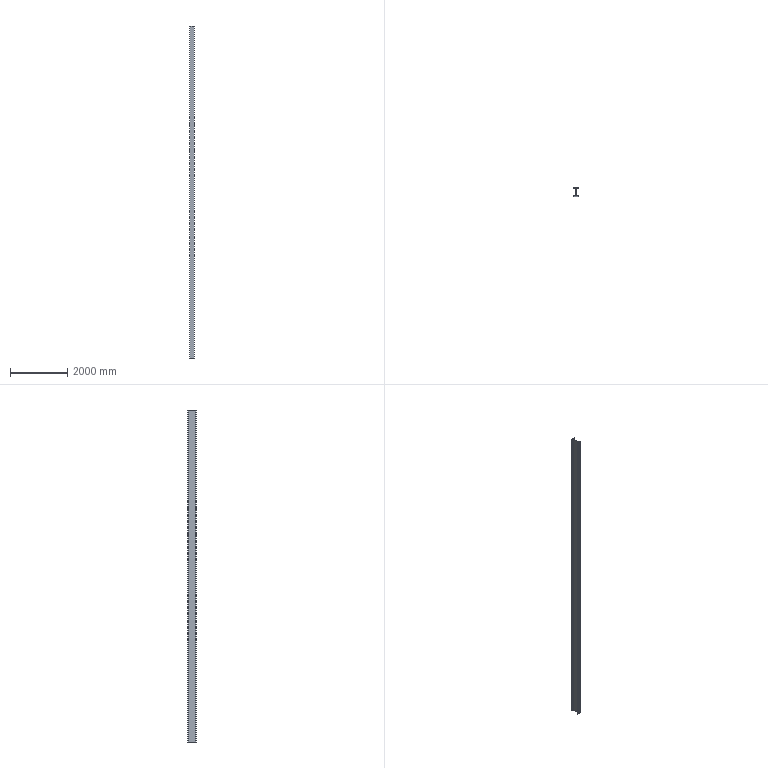Part | SolidWorks | features Extrusion 1 | 1 solid | 18 faces | box 150 x 300 x 11647 mm | volume 54485491 mm3 | plane 14 | cylinder 4 | commonest cylinder face diameters 26 x4
STEP:
#1=CARTESIAN_POINT('',(-75.,9.,0.));
#2=VERTEX_POINT('',#1);
#3=CARTESIAN_POINT('',(-75.,0.,0.));
#4=VERTEX_POINT('',#3);
#5=CARTESIAN_POINT('',(-75.,0.,0.));
#6=DIRECTION('',(0.,-1.,0.));
#7=VECTOR('',#6,1000.);
#8=LINE('',#5,#7);
#9=EDGE_CURVE('',#2,#4,#8,.T.);
#10=ORIENTED_EDGE('',*,*,#9,.T.);
#11=CARTESIAN_POINT('',(-75.,0.,11647.));
#12=VERTEX_POINT('',#11);
#13=CARTESIAN_POINT('',(-75.,0.,11647.));
#14=DIRECTION('',(0.,0.,-1.));
#15=VECTOR('',#14,1000.);
#16=LINE('',#13,#15);
#17=EDGE_CURVE('',#12,#4,#16,.T.);
#18=ORIENTED_EDGE('',*,*,#17,.F.);
#19=CARTESIAN_POINT('',(-75.,9.,11647.));
#20=VERTEX_POINT('',#19);
#21=CARTESIAN_POINT('',(-75.,0.,11647.));
#22=DIRECTION('',(0.,-1.,0.));
#23=VECTOR('',#22,1000.);
#24=LINE('',#21,#23);
#25=EDGE_CURVE('',#20,#12,#24,.T.);
#26=ORIENTED_EDGE('',*,*,#25,.F.);
#27=CARTESIAN_POINT('',(-75.,9.,11647.));
#28=DIRECTION('',(0.,0.,-1.));
#29=VECTOR('',#28,1000.);
#30=LINE('',#27,#29);
#31=EDGE_CURVE('',#20,#2,#30,.T.);
#32=ORIENTED_EDGE('',*,*,#31,.T.);
#33=EDGE_LOOP('',(#10,#18,#26,#32));
#34=FACE_OUTER_BOUND('',#33,.T.);
#35=CARTESIAN_POINT('',(-75.,0.,11647.));
#36=DIRECTION('',(1.,0.,0.));
#37=DIRECTION('',(0.,0.,-1.));
#38=AXIS2_PLACEMENT_3D('',#35,#36,#37);
#39=PLANE('',#38);
#40=ADVANCED_FACE('',(#34),#39,.F.);
#41=CARTESIAN_POINT('',(75.,0.,0.));
#42=VERTEX_POINT('',#41);
#43=CARTESIAN_POINT('',(75.,0.,0.));
#44=DIRECTION('',(1.,0.,0.));
#45=VECTOR('',#44,1000.);
#46=LINE('',#43,#45);
#47=EDGE_CURVE('',#4,#42,#46,.T.);
#48=ORIENTED_EDGE('',*,*,#47,.T.);
#49=CARTESIAN_POINT('',(75.,0.,11647.));
#50=VERTEX_POINT('',#49);
#51=CARTESIAN_POINT('',(75.,0.,11647.));
#52=DIRECTION('',(0.,0.,-1.));
#53=VECTOR('',#52,1000.);
#54=LINE('',#51,#53);
#55=EDGE_CURVE('',#50,#42,#54,.T.);
#56=ORIENTED_EDGE('',*,*,#55,.F.);
#57=CARTESIAN_POINT('',(75.,0.,11647.));
#58=DIRECTION('',(1.,0.,0.));
#59=VECTOR('',#58,1000.);
#60=LINE('',#57,#59);
#61=EDGE_CURVE('',#12,#50,#60,.T.);
#62=ORIENTED_EDGE('',*,*,#61,.F.);
#63=ORIENTED_EDGE('',*,*,#17,.T.);
#64=EDGE_LOOP('',(#48,#56,#62,#63));
#65=FACE_OUTER_BOUND('',#64,.T.);
#66=CARTESIAN_POINT('',(75.,0.,11647.));
#67=DIRECTION('',(0.,1.,0.));
#68=DIRECTION('',(-1.,0.,0.));
#69=AXIS2_PLACEMENT_3D('',#66,#67,#68);
#70=PLANE('',#69);
#71=ADVANCED_FACE('',(#65),#70,.F.);
#72=CARTESIAN_POINT('',(75.,9.,0.));
#73=VERTEX_POINT('',#72);
#74=CARTESIAN_POINT('',(75.,0.,0.));
#75=DIRECTION('',(0.,1.,0.));
#76=VECTOR('',#75,1000.);
#77=LINE('',#74,#76);
#78=EDGE_CURVE('',#42,#73,#77,.T.);
#79=ORIENTED_EDGE('',*,*,#78,.T.);
#80=CARTESIAN_POINT('',(75.,9.,11647.));
#81=VERTEX_POINT('',#80);
#82=CARTESIAN_POINT('',(75.,9.,11647.));
#83=DIRECTION('',(0.,0.,-1.));
#84=VECTOR('',#83,1000.);
#85=LINE('',#82,#84);
#86=EDGE_CURVE('',#81,#73,#85,.T.);
#87=ORIENTED_EDGE('',*,*,#86,.F.);
#88=CARTESIAN_POINT('',(75.,0.,11647.));
#89=DIRECTION('',(0.,1.,0.));
#90=VECTOR('',#89,1000.);
#91=LINE('',#88,#90);
#92=EDGE_CURVE('',#50,#81,#91,.T.);
#93=ORIENTED_EDGE('',*,*,#92,.F.);
#94=ORIENTED_EDGE('',*,*,#55,.T.);
#95=EDGE_LOOP('',(#79,#87,#93,#94));
#96=FACE_OUTER_BOUND('',#95,.T.);
#97=CARTESIAN_POINT('',(75.,0.,11647.));
#98=DIRECTION('',(-1.,0.,0.));
#99=DIRECTION('',(0.,0.,1.));
#100=AXIS2_PLACEMENT_3D('',#97,#98,#99);
#101=PLANE('',#100);
#102=ADVANCED_FACE('',(#96),#101,.F.);
#103=CARTESIAN_POINT('',(16.25,9.,0.));
#104=VERTEX_POINT('',#103);
#105=CARTESIAN_POINT('',(75.,9.,0.));
#106=DIRECTION('',(-1.,0.,0.));
#107=VECTOR('',#106,1000.);
#108=LINE('',#105,#107);
#109=EDGE_CURVE('',#73,#104,#108,.T.);
#110=ORIENTED_EDGE('',*,*,#109,.T.);
#111=CARTESIAN_POINT('',(16.25,9.,11647.));
#112=VERTEX_POINT('',#111);
#113=CARTESIAN_POINT('',(16.25,9.,11647.));
#114=DIRECTION('',(0.,0.,-1.));
#115=VECTOR('',#114,1000.);
#116=LINE('',#113,#115);
#117=EDGE_CURVE('',#112,#104,#116,.T.);
#118=ORIENTED_EDGE('',*,*,#117,.F.);
#119=CARTESIAN_POINT('',(75.,9.,11647.));
#120=DIRECTION('',(-1.,0.,0.));
#121=VECTOR('',#120,1000.);
#122=LINE('',#119,#121);
#123=EDGE_CURVE('',#81,#112,#122,.T.);
#124=ORIENTED_EDGE('',*,*,#123,.F.);
#125=ORIENTED_EDGE('',*,*,#86,.T.);
#126=EDGE_LOOP('',(#110,#118,#124,#125));
#127=FACE_OUTER_BOUND('',#126,.T.);
#128=CARTESIAN_POINT('',(75.,9.,11647.));
#129=DIRECTION('',(0.,-1.,0.));
#130=DIRECTION('',(1.,0.,0.));
#131=AXIS2_PLACEMENT_3D('',#128,#129,#130);
#132=PLANE('',#131);
#133=ADVANCED_FACE('',(#127),#132,.F.);
#134=CARTESIAN_POINT('',(3.25,22.,0.));
#135=VERTEX_POINT('',#134);
#136=CARTESIAN_POINT('',(16.25,22.,0.));
#137=DIRECTION('',(0.,0.,-1.));
#138=DIRECTION('',(-1.,0.,0.));
#139=AXIS2_PLACEMENT_3D('',#136,#137,#138);
#140=CIRCLE('',#139,13.);
#141=EDGE_CURVE('',#104,#135,#140,.T.);
#142=ORIENTED_EDGE('',*,*,#141,.T.);
#143=CARTESIAN_POINT('',(3.25,22.,11647.));
#144=VERTEX_POINT('',#143);
#145=CARTESIAN_POINT('',(3.25,22.,11647.));
#146=DIRECTION('',(0.,0.,-1.));
#147=VECTOR('',#146,1000.);
#148=LINE('',#145,#147);
#149=EDGE_CURVE('',#144,#135,#148,.T.);
#150=ORIENTED_EDGE('',*,*,#149,.F.);
#151=CARTESIAN_POINT('',(16.25,22.,11647.));
#152=DIRECTION('',(0.,0.,-1.));
#153=DIRECTION('',(-1.,0.,0.));
#154=AXIS2_PLACEMENT_3D('',#151,#152,#153);
#155=CIRCLE('',#154,13.);
#156=EDGE_CURVE('',#112,#144,#155,.T.);
#157=ORIENTED_EDGE('',*,*,#156,.F.);
#158=ORIENTED_EDGE('',*,*,#117,.T.);
#159=EDGE_LOOP('',(#142,#150,#157,#158));
#160=FACE_OUTER_BOUND('',#159,.T.);
#161=CARTESIAN_POINT('',(16.25,22.,11647.));
#162=DIRECTION('',(0.,0.,-1.));
#163=DIRECTION('',(-1.,0.,0.));
#164=AXIS2_PLACEMENT_3D('',#161,#162,#163);
#165=CYLINDRICAL_SURFACE('',#164,13.);
#166=ADVANCED_FACE('',(#160),#165,.F.);
#167=CARTESIAN_POINT('',(3.25,278.,0.));
#168=VERTEX_POINT('',#167);
#169=CARTESIAN_POINT('',(3.25,22.,0.));
#170=DIRECTION('',(0.,1.,0.));
#171=VECTOR('',#170,1000.);
#172=LINE('',#169,#171);
#173=EDGE_CURVE('',#135,#168,#172,.T.);
#174=ORIENTED_EDGE('',*,*,#173,.T.);
#175=CARTESIAN_POINT('',(3.25,278.,11647.));
#176=VERTEX_POINT('',#175);
#177=CARTESIAN_POINT('',(3.25,278.,11647.));
#178=DIRECTION('',(0.,0.,-1.));
#179=VECTOR('',#178,1000.);
#180=LINE('',#177,#179);
#181=EDGE_CURVE('',#176,#168,#180,.T.);
#182=ORIENTED_EDGE('',*,*,#181,.F.);
#183=CARTESIAN_POINT('',(3.25,22.,11647.));
#184=DIRECTION('',(0.,1.,0.));
#185=VECTOR('',#184,1000.);
#186=LINE('',#183,#185);
#187=EDGE_CURVE('',#144,#176,#186,.T.);
#188=ORIENTED_EDGE('',*,*,#187,.F.);
#189=ORIENTED_EDGE('',*,*,#149,.T.);
#190=EDGE_LOOP('',(#174,#182,#188,#189));
#191=FACE_OUTER_BOUND('',#190,.T.);
#192=CARTESIAN_POINT('',(3.25,22.,11647.));
#193=DIRECTION('',(-1.,0.,0.));
#194=DIRECTION('',(0.,0.,1.));
#195=AXIS2_PLACEMENT_3D('',#192,#193,#194);
#196=PLANE('',#195);
#197=ADVANCED_FACE('',(#191),#196,.F.);
#198=CARTESIAN_POINT('',(16.25,291.,0.));
#199=VERTEX_POINT('',#198);
#200=CARTESIAN_POINT('',(16.25,278.,0.));
#201=DIRECTION('',(0.,0.,-1.));
#202=DIRECTION('',(-1.,0.,0.));
#203=AXIS2_PLACEMENT_3D('',#200,#201,#202);
#204=CIRCLE('',#203,13.);
#205=EDGE_CURVE('',#168,#199,#204,.T.);
#206=ORIENTED_EDGE('',*,*,#205,.T.);
#207=CARTESIAN_POINT('',(16.25,291.,11647.));
#208=VERTEX_POINT('',#207);
#209=CARTESIAN_POINT('',(16.25,291.,11647.));
#210=DIRECTION('',(0.,0.,-1.));
#211=VECTOR('',#210,1000.);
#212=LINE('',#209,#211);
#213=EDGE_CURVE('',#208,#199,#212,.T.);
#214=ORIENTED_EDGE('',*,*,#213,.F.);
#215=CARTESIAN_POINT('',(16.25,278.,11647.));
#216=DIRECTION('',(0.,0.,-1.));
#217=DIRECTION('',(-1.,0.,0.));
#218=AXIS2_PLACEMENT_3D('',#215,#216,#217);
#219=CIRCLE('',#218,13.);
#220=EDGE_CURVE('',#176,#208,#219,.T.);
#221=ORIENTED_EDGE('',*,*,#220,.F.);
#222=ORIENTED_EDGE('',*,*,#181,.T.);
#223=EDGE_LOOP('',(#206,#214,#221,#222));
#224=FACE_OUTER_BOUND('',#223,.T.);
#225=CARTESIAN_POINT('',(16.25,278.,11647.));
#226=DIRECTION('',(0.,0.,-1.));
#227=DIRECTION('',(-1.,0.,0.));
#228=AXIS2_PLACEMENT_3D('',#225,#226,#227);
#229=CYLINDRICAL_SURFACE('',#228,13.);
#230=ADVANCED_FACE('',(#224),#229,.F.);
#231=CARTESIAN_POINT('',(75.,291.,0.));
#232=VERTEX_POINT('',#231);
#233=CARTESIAN_POINT('',(16.25,291.,0.));
#234=DIRECTION('',(1.,0.,0.));
#235=VECTOR('',#234,1000.);
#236=LINE('',#233,#235);
#237=EDGE_CURVE('',#199,#232,#236,.T.);
#238=ORIENTED_EDGE('',*,*,#237,.T.);
#239=CARTESIAN_POINT('',(75.,291.,11647.));
#240=VERTEX_POINT('',#239);
#241=CARTESIAN_POINT('',(75.,291.,11647.));
#242=DIRECTION('',(0.,0.,-1.));
#243=VECTOR('',#242,1000.);
#244=LINE('',#241,#243);
#245=EDGE_CURVE('',#240,#232,#244,.T.);
#246=ORIENTED_EDGE('',*,*,#245,.F.);
#247=CARTESIAN_POINT('',(16.25,291.,11647.));
#248=DIRECTION('',(1.,0.,0.));
#249=VECTOR('',#248,1000.);
#250=LINE('',#247,#249);
#251=EDGE_CURVE('',#208,#240,#250,.T.);
#252=ORIENTED_EDGE('',*,*,#251,.F.);
#253=ORIENTED_EDGE('',*,*,#213,.T.);
#254=EDGE_LOOP('',(#238,#246,#252,#253));
#255=FACE_OUTER_BOUND('',#254,.T.);
#256=CARTESIAN_POINT('',(16.25,291.,11647.));
#257=DIRECTION('',(0.,1.,0.));
#258=DIRECTION('',(-1.,0.,0.));
#259=AXIS2_PLACEMENT_3D('',#256,#257,#258);
#260=PLANE('',#259);
#261=ADVANCED_FACE('',(#255),#260,.F.);
#262=CARTESIAN_POINT('',(75.,300.,0.));
#263=VERTEX_POINT('',#262);
#264=CARTESIAN_POINT('',(75.,291.,0.));
#265=DIRECTION('',(0.,1.,0.));
#266=VECTOR('',#265,1000.);
#267=LINE('',#264,#266);
#268=EDGE_CURVE('',#232,#263,#267,.T.);
#269=ORIENTED_EDGE('',*,*,#268,.T.);
#270=CARTESIAN_POINT('',(75.,300.,11647.));
#271=VERTEX_POINT('',#270);
#272=CARTESIAN_POINT('',(75.,300.,11647.));
#273=DIRECTION('',(0.,0.,-1.));
#274=VECTOR('',#273,1000.);
#275=LINE('',#272,#274);
#276=EDGE_CURVE('',#271,#263,#275,.T.);
#277=ORIENTED_EDGE('',*,*,#276,.F.);
#278=CARTESIAN_POINT('',(75.,291.,11647.));
#279=DIRECTION('',(0.,1.,0.));
#280=VECTOR('',#279,1000.);
#281=LINE('',#278,#280);
#282=EDGE_CURVE('',#240,#271,#281,.T.);
#283=ORIENTED_EDGE('',*,*,#282,.F.);
#284=ORIENTED_EDGE('',*,*,#245,.T.);
#285=EDGE_LOOP('',(#269,#277,#283,#284));
#286=FACE_OUTER_BOUND('',#285,.T.);
#287=CARTESIAN_POINT('',(75.,291.,11647.));
#288=DIRECTION('',(-1.,0.,0.));
#289=DIRECTION('',(0.,-1.,0.));
#290=AXIS2_PLACEMENT_3D('',#287,#288,#289);
#291=PLANE('',#290);
#292=ADVANCED_FACE('',(#286),#291,.F.);
#293=CARTESIAN_POINT('',(-75.,300.,0.));
#294=VERTEX_POINT('',#293);
#295=CARTESIAN_POINT('',(-75.,300.,0.));
#296=DIRECTION('',(-1.,0.,0.));
#297=VECTOR('',#296,1000.);
#298=LINE('',#295,#297);
#299=EDGE_CURVE('',#263,#294,#298,.T.);
#300=ORIENTED_EDGE('',*,*,#299,.T.);
#301=CARTESIAN_POINT('',(-75.,300.,11647.));
#302=VERTEX_POINT('',#301);
#303=CARTESIAN_POINT('',(-75.,300.,11647.));
#304=DIRECTION('',(0.,0.,-1.));
#305=VECTOR('',#304,1000.);
#306=LINE('',#303,#305);
#307=EDGE_CURVE('',#302,#294,#306,.T.);
#308=ORIENTED_EDGE('',*,*,#307,.F.);
#309=CARTESIAN_POINT('',(-75.,300.,11647.));
#310=DIRECTION('',(-1.,0.,0.));
#311=VECTOR('',#310,1000.);
#312=LINE('',#309,#311);
#313=EDGE_CURVE('',#271,#302,#312,.T.);
#314=ORIENTED_EDGE('',*,*,#313,.F.);
#315=ORIENTED_EDGE('',*,*,#276,.T.);
#316=EDGE_LOOP('',(#300,#308,#314,#315));
#317=FACE_OUTER_BOUND('',#316,.T.);
#318=CARTESIAN_POINT('',(-75.,300.,11647.));
#319=DIRECTION('',(0.,-1.,0.));
#320=DIRECTION('',(0.,0.,-1.));
#321=AXIS2_PLACEMENT_3D('',#318,#319,#320);
#322=PLANE('',#321);
#323=ADVANCED_FACE('',(#317),#322,.F.);
#324=CARTESIAN_POINT('',(-75.,291.,0.));
#325=VERTEX_POINT('',#324);
#326=CARTESIAN_POINT('',(-75.,291.,0.));
#327=DIRECTION('',(0.,-1.,0.));
#328=VECTOR('',#327,1000.);
#329=LINE('',#326,#328);
#330=EDGE_CURVE('',#294,#325,#329,.T.);
#331=ORIENTED_EDGE('',*,*,#330,.T.);
#332=CARTESIAN_POINT('',(-75.,291.,11647.));
#333=VERTEX_POINT('',#332);
#334=CARTESIAN_POINT('',(-75.,291.,11647.));
#335=DIRECTION('',(0.,0.,-1.));
#336=VECTOR('',#335,1000.);
#337=LINE('',#334,#336);
#338=EDGE_CURVE('',#333,#325,#337,.T.);
#339=ORIENTED_EDGE('',*,*,#338,.F.);
#340=CARTESIAN_POINT('',(-75.,291.,11647.));
#341=DIRECTION('',(0.,-1.,0.));
#342=VECTOR('',#341,1000.);
#343=LINE('',#340,#342);
#344=EDGE_CURVE('',#302,#333,#343,.T.);
#345=ORIENTED_EDGE('',*,*,#344,.F.);
#346=ORIENTED_EDGE('',*,*,#307,.T.);
#347=EDGE_LOOP('',(#331,#339,#345,#346));
#348=FACE_OUTER_BOUND('',#347,.T.);
#349=CARTESIAN_POINT('',(-75.,291.,11647.));
#350=DIRECTION('',(1.,0.,0.));
#351=DIRECTION('',(0.,1.,0.));
#352=AXIS2_PLACEMENT_3D('',#349,#350,#351);
#353=PLANE('',#352);
#354=ADVANCED_FACE('',(#348),#353,.F.);
#355=CARTESIAN_POINT('',(-16.25,291.,0.));
#356=VERTEX_POINT('',#355);
#357=CARTESIAN_POINT('',(-16.25,291.,0.));
#358=DIRECTION('',(1.,0.,0.));
#359=VECTOR('',#358,1000.);
#360=LINE('',#357,#359);
#361=EDGE_CURVE('',#325,#356,#360,.T.);
#362=ORIENTED_EDGE('',*,*,#361,.T.);
#363=CARTESIAN_POINT('',(-16.25,291.,11647.));
#364=VERTEX_POINT('',#363);
#365=CARTESIAN_POINT('',(-16.25,291.,11647.));
#366=DIRECTION('',(0.,0.,-1.));
#367=VECTOR('',#366,1000.);
#368=LINE('',#365,#367);
#369=EDGE_CURVE('',#364,#356,#368,.T.);
#370=ORIENTED_EDGE('',*,*,#369,.F.);
#371=CARTESIAN_POINT('',(-16.25,291.,11647.));
#372=DIRECTION('',(1.,0.,0.));
#373=VECTOR('',#372,1000.);
#374=LINE('',#371,#373);
#375=EDGE_CURVE('',#333,#364,#374,.T.);
#376=ORIENTED_EDGE('',*,*,#375,.F.);
#377=ORIENTED_EDGE('',*,*,#338,.T.);
#378=EDGE_LOOP('',(#362,#370,#376,#377));
#379=FACE_OUTER_BOUND('',#378,.T.);
#380=CARTESIAN_POINT('',(-16.25,291.,11647.));
#381=DIRECTION('',(0.,1.,0.));
#382=DIRECTION('',(-1.,0.,0.));
#383=AXIS2_PLACEMENT_3D('',#380,#381,#382);
#384=PLANE('',#383);
#385=ADVANCED_FACE('',(#379),#384,.F.);
#386=CARTESIAN_POINT('',(-3.25,278.,0.));
#387=VERTEX_POINT('',#386);
#388=CARTESIAN_POINT('',(-16.25,278.,0.));
#389=DIRECTION('',(0.,0.,-1.));
#390=DIRECTION('',(1.,0.,0.));
#391=AXIS2_PLACEMENT_3D('',#388,#389,#390);
#392=CIRCLE('',#391,13.);
#393=EDGE_CURVE('',#356,#387,#392,.T.);
#394=ORIENTED_EDGE('',*,*,#393,.T.);
#395=CARTESIAN_POINT('',(-3.25,278.,11647.));
#396=VERTEX_POINT('',#395);
#397=CARTESIAN_POINT('',(-3.25,278.,11647.));
#398=DIRECTION('',(0.,0.,-1.));
#399=VECTOR('',#398,1000.);
#400=LINE('',#397,#399);
#401=EDGE_CURVE('',#396,#387,#400,.T.);
#402=ORIENTED_EDGE('',*,*,#401,.F.);
#403=CARTESIAN_POINT('',(-16.25,278.,11647.));
#404=DIRECTION('',(0.,0.,-1.));
#405=DIRECTION('',(1.,0.,0.));
#406=AXIS2_PLACEMENT_3D('',#403,#404,#405);
#407=CIRCLE('',#406,13.);
#408=EDGE_CURVE('',#364,#396,#407,.T.);
#409=ORIENTED_EDGE('',*,*,#408,.F.);
#410=ORIENTED_EDGE('',*,*,#369,.T.);
#411=EDGE_LOOP('',(#394,#402,#409,#410));
#412=FACE_OUTER_BOUND('',#411,.T.);
#413=CARTESIAN_POINT('',(-16.25,278.,11647.));
#414=DIRECTION('',(0.,0.,-1.));
#415=DIRECTION('',(-1.,0.,0.));
#416=AXIS2_PLACEMENT_3D('',#413,#414,#415);
#417=CYLINDRICAL_SURFACE('',#416,13.);
#418=ADVANCED_FACE('',(#412),#417,.F.);
#419=CARTESIAN_POINT('',(-3.25,22.,0.));
#420=VERTEX_POINT('',#419);
#421=CARTESIAN_POINT('',(-3.25,22.,0.));
#422=DIRECTION('',(0.,-1.,0.));
#423=VECTOR('',#422,1000.);
#424=LINE('',#421,#423);
#425=EDGE_CURVE('',#387,#420,#424,.T.);
#426=ORIENTED_EDGE('',*,*,#425,.T.);
#427=CARTESIAN_POINT('',(-3.25,22.,11647.));
#428=VERTEX_POINT('',#427);
#429=CARTESIAN_POINT('',(-3.25,22.,11647.));
#430=DIRECTION('',(0.,0.,-1.));
#431=VECTOR('',#430,1000.);
#432=LINE('',#429,#431);
#433=EDGE_CURVE('',#428,#420,#432,.T.);
#434=ORIENTED_EDGE('',*,*,#433,.F.);
#435=CARTESIAN_POINT('',(-3.25,22.,11647.));
#436=DIRECTION('',(0.,-1.,0.));
#437=VECTOR('',#436,1000.);
#438=LINE('',#435,#437);
#439=EDGE_CURVE('',#396,#428,#438,.T.);
#440=ORIENTED_EDGE('',*,*,#439,.F.);
#441=ORIENTED_EDGE('',*,*,#401,.T.);
#442=EDGE_LOOP('',(#426,#434,#440,#441));
#443=FACE_OUTER_BOUND('',#442,.T.);
#444=CARTESIAN_POINT('',(-3.25,22.,11647.));
#445=DIRECTION('',(1.,0.,0.));
#446=DIRECTION('',(0.,0.,-1.));
#447=AXIS2_PLACEMENT_3D('',#444,#445,#446);
#448=PLANE('',#447);
#449=ADVANCED_FACE('',(#443),#448,.F.);
#450=CARTESIAN_POINT('',(-16.25,9.,0.));
#451=VERTEX_POINT('',#450);
#452=CARTESIAN_POINT('',(-16.25,22.,0.));
#453=DIRECTION('',(0.,0.,-1.));
#454=DIRECTION('',(-1.,0.,0.));
#455=AXIS2_PLACEMENT_3D('',#452,#453,#454);
#456=CIRCLE('',#455,13.);
#457=EDGE_CURVE('',#420,#451,#456,.T.);
#458=ORIENTED_EDGE('',*,*,#457,.T.);
#459=CARTESIAN_POINT('',(-16.25,9.,11647.));
#460=VERTEX_POINT('',#459);
#461=CARTESIAN_POINT('',(-16.25,9.,11647.));
#462=DIRECTION('',(0.,0.,-1.));
#463=VECTOR('',#462,1000.);
#464=LINE('',#461,#463);
#465=EDGE_CURVE('',#460,#451,#464,.T.);
#466=ORIENTED_EDGE('',*,*,#465,.F.);
#467=CARTESIAN_POINT('',(-16.25,22.,11647.));
#468=DIRECTION('',(0.,0.,-1.));
#469=DIRECTION('',(-1.,0.,0.));
#470=AXIS2_PLACEMENT_3D('',#467,#468,#469);
#471=CIRCLE('',#470,13.);
#472=EDGE_CURVE('',#428,#460,#471,.T.);
#473=ORIENTED_EDGE('',*,*,#472,.F.);
#474=ORIENTED_EDGE('',*,*,#433,.T.);
#475=EDGE_LOOP('',(#458,#466,#473,#474));
#476=FACE_OUTER_BOUND('',#475,.T.);
#477=CARTESIAN_POINT('',(-16.25,22.,11647.));
#478=DIRECTION('',(0.,0.,-1.));
#479=DIRECTION('',(-1.,0.,0.));
#480=AXIS2_PLACEMENT_3D('',#477,#478,#479);
#481=CYLINDRICAL_SURFACE('',#480,13.);
#482=ADVANCED_FACE('',(#476),#481,.F.);
#483=CARTESIAN_POINT('',(-75.,9.,0.));
#484=DIRECTION('',(-1.,0.,0.));
#485=VECTOR('',#484,1000.);
#486=LINE('',#483,#485);
#487=EDGE_CURVE('',#451,#2,#486,.T.);
#488=ORIENTED_EDGE('',*,*,#487,.T.);
#489=ORIENTED_EDGE('',*,*,#31,.F.);
#490=CARTESIAN_POINT('',(-75.,9.,11647.));
#491=DIRECTION('',(-1.,0.,0.));
#492=VECTOR('',#491,1000.);
#493=LINE('',#490,#492);
#494=EDGE_CURVE('',#460,#20,#493,.T.);
#495=ORIENTED_EDGE('',*,*,#494,.F.);
#496=ORIENTED_EDGE('',*,*,#465,.T.);
#497=EDGE_LOOP('',(#488,#489,#495,#496));
#498=FACE_OUTER_BOUND('',#497,.T.);
#499=CARTESIAN_POINT('',(-75.,9.,11647.));
#500=DIRECTION('',(0.,-1.,0.));
#501=DIRECTION('',(1.,0.,0.));
#502=AXIS2_PLACEMENT_3D('',#499,#500,#501);
#503=PLANE('',#502);
#504=ADVANCED_FACE('',(#498),#503,.F.);
#505=ORIENTED_EDGE('',*,*,#25,.T.);
#506=ORIENTED_EDGE('',*,*,#61,.T.);
#507=ORIENTED_EDGE('',*,*,#92,.T.);
#508=ORIENTED_EDGE('',*,*,#123,.T.);
#509=ORIENTED_EDGE('',*,*,#156,.T.);
#510=ORIENTED_EDGE('',*,*,#187,.T.);
#511=ORIENTED_EDGE('',*,*,#220,.T.);
#512=ORIENTED_EDGE('',*,*,#251,.T.);
#513=ORIENTED_EDGE('',*,*,#282,.T.);
#514=ORIENTED_EDGE('',*,*,#313,.T.);
#515=ORIENTED_EDGE('',*,*,#344,.T.);
#516=ORIENTED_EDGE('',*,*,#375,.T.);
#517=ORIENTED_EDGE('',*,*,#408,.T.);
#518=ORIENTED_EDGE('',*,*,#439,.T.);
#519=ORIENTED_EDGE('',*,*,#472,.T.);
#520=ORIENTED_EDGE('',*,*,#494,.T.);
#521=EDGE_LOOP('',(#505,#506,#507,#508,#509,#510,#511,#512,#513,#514,#515,#516,#517,#518,#519,#520));
#522=FACE_OUTER_BOUND('',#521,.T.);
#523=CARTESIAN_POINT('',(-16.25,22.,11647.));
#524=DIRECTION('',(0.,0.,-1.));
#525=DIRECTION('',(-1.,0.,0.));
#526=AXIS2_PLACEMENT_3D('',#523,#524,#525);
#527=PLANE('',#526);
#528=ADVANCED_FACE('',(#522),#527,.F.);
#529=ORIENTED_EDGE('',*,*,#9,.F.);
#530=ORIENTED_EDGE('',*,*,#487,.F.);
#531=ORIENTED_EDGE('',*,*,#457,.F.);
#532=ORIENTED_EDGE('',*,*,#425,.F.);
#533=ORIENTED_EDGE('',*,*,#393,.F.);
#534=ORIENTED_EDGE('',*,*,#361,.F.);
#535=ORIENTED_EDGE('',*,*,#330,.F.);
#536=ORIENTED_EDGE('',*,*,#299,.F.);
#537=ORIENTED_EDGE('',*,*,#268,.F.);
#538=ORIENTED_EDGE('',*,*,#237,.F.);
#539=ORIENTED_EDGE('',*,*,#205,.F.);
#540=ORIENTED_EDGE('',*,*,#173,.F.);
#541=ORIENTED_EDGE('',*,*,#141,.F.);
#542=ORIENTED_EDGE('',*,*,#109,.F.);
#543=ORIENTED_EDGE('',*,*,#78,.F.);
#544=ORIENTED_EDGE('',*,*,#47,.F.);
#545=EDGE_LOOP('',(#529,#530,#531,#532,#533,#534,#535,#536,#537,#538,#539,#540,#541,#542,#543,#544));
#546=FACE_OUTER_BOUND('',#545,.T.);
#547=CARTESIAN_POINT('',(-16.25,22.,0.));
#548=DIRECTION('',(0.,0.,-1.));
#549=DIRECTION('',(-1.,0.,0.));
#550=AXIS2_PLACEMENT_3D('',#547,#548,#549);
#551=PLANE('',#550);
#552=ADVANCED_FACE('',(#546),#551,.T.);
#553=CLOSED_SHELL('',(#40,#71,#102,#133,#166,#197,#230,#261,#292,#323,#354,#385,#418,#449,#482,#504,#528,#552));
#554=MANIFOLD_SOLID_BREP('',#553);
#555=CARTESIAN_POINT('',(0.,0.,0.));
#556=DIRECTION('',(0.,0.,1.));
#557=DIRECTION('',(1.,0.,0.));
#558=AXIS2_PLACEMENT_3D('',#555,#556,#557);
#559=(LENGTH_UNIT()NAMED_UNIT(*)SI_UNIT(.MILLI.,.METRE.));
#560=UNCERTAINTY_MEASURE_WITH_UNIT(LENGTH_MEASURE(0.00001),#559,'','');
#561=(NAMED_UNIT(*)PLANE_ANGLE_UNIT()SI_UNIT($,.RADIAN.));
#562=(NAMED_UNIT(*)SI_UNIT($,.STERADIAN.)SOLID_ANGLE_UNIT());
#563=(GEOMETRIC_REPRESENTATION_CONTEXT(3)GLOBAL_UNCERTAINTY_ASSIGNED_CONTEXT((#560))GLOBAL_UNIT_ASSIGNED_CONTEXT((#559,#561,#562))REPRESENTATION_CONTEXT('',''));
#564=ADVANCED_BREP_SHAPE_REPRESENTATION('',(#554,#558),#563);